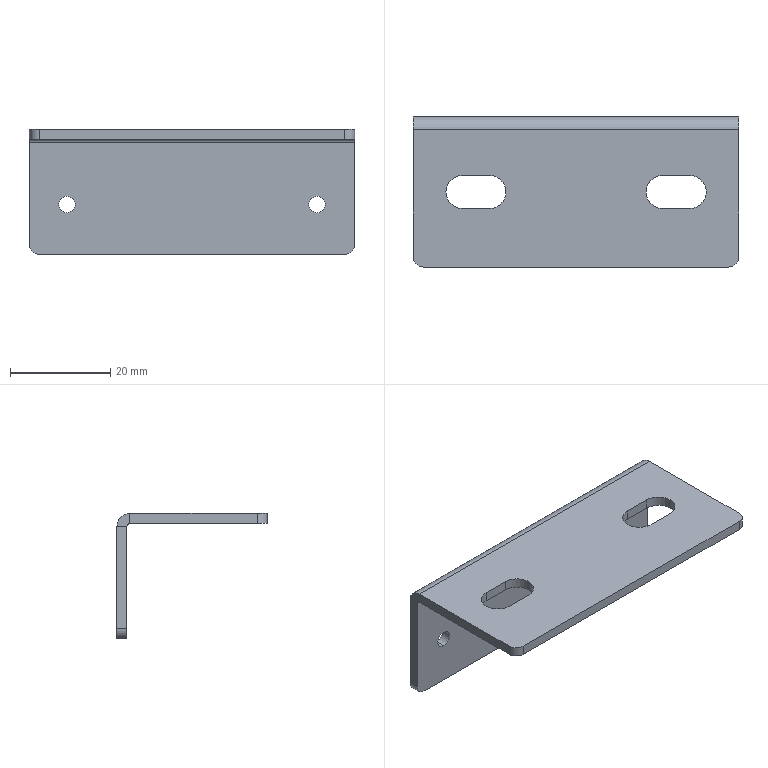Part | STEP file | Cover Plate Adapter Plate | 1 solid | 32 faces | box 65 x 30 x 25 mm | volume 6480 mm3 | cylinder 16 | plane 16 | commonest cylinder face diameters 6.6 x6 3.3 x4 4 x4 1.2 x1 5.2 x1